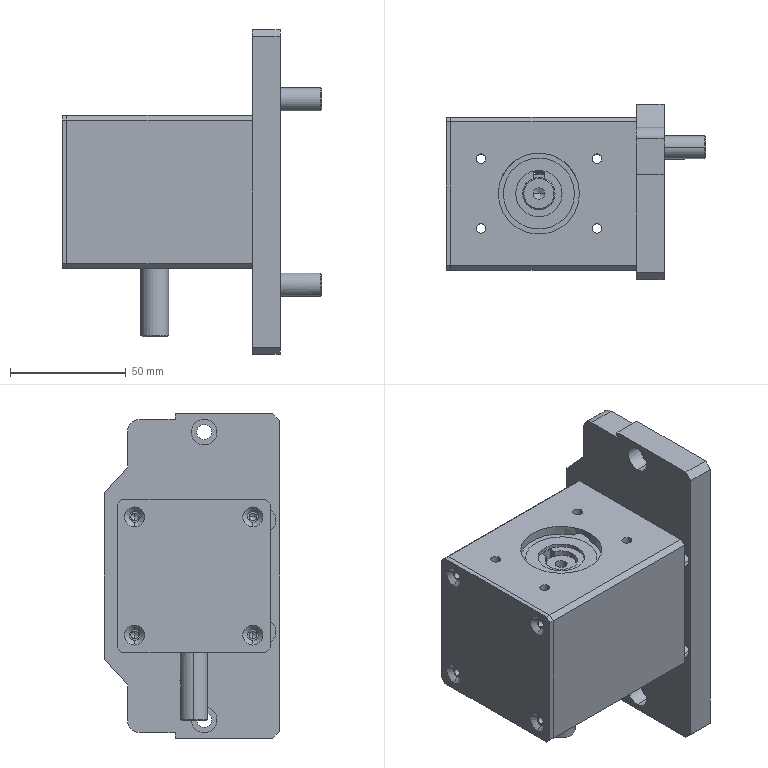Part | NX | features BREP 9 | 9 solids | 254 faces | box 112 x 75.5 x 140 mm | volume 346722 mm3 | cylinder 125 | plane 86 | cone 43 | commonest cylinder face diameters 4.2 x16 6.5 x14 3.3 x12 8 x12 5 x10 10 x10